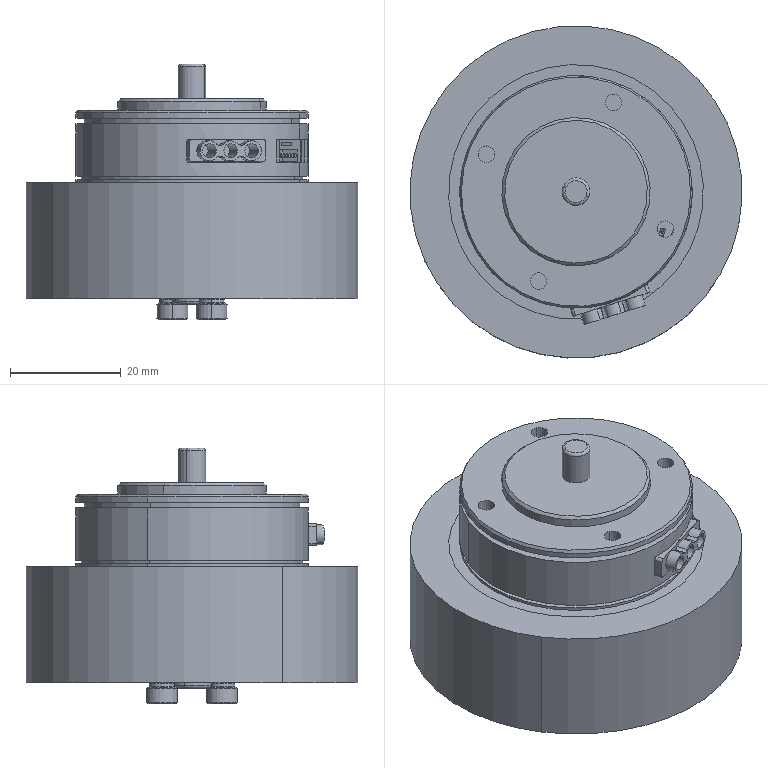Part | SolidWorks | 12 solids | 606 faces | box 60 x 60 x 46.2 mm | volume 74410 mm3 | plane 294 | cylinder 179 | spline 89 | cone 24 | torus 20 | commonest cylinder face diameters 1.4 x30 3 x24 0.2 x14 0.786 x14 36.56 x13 2 x8